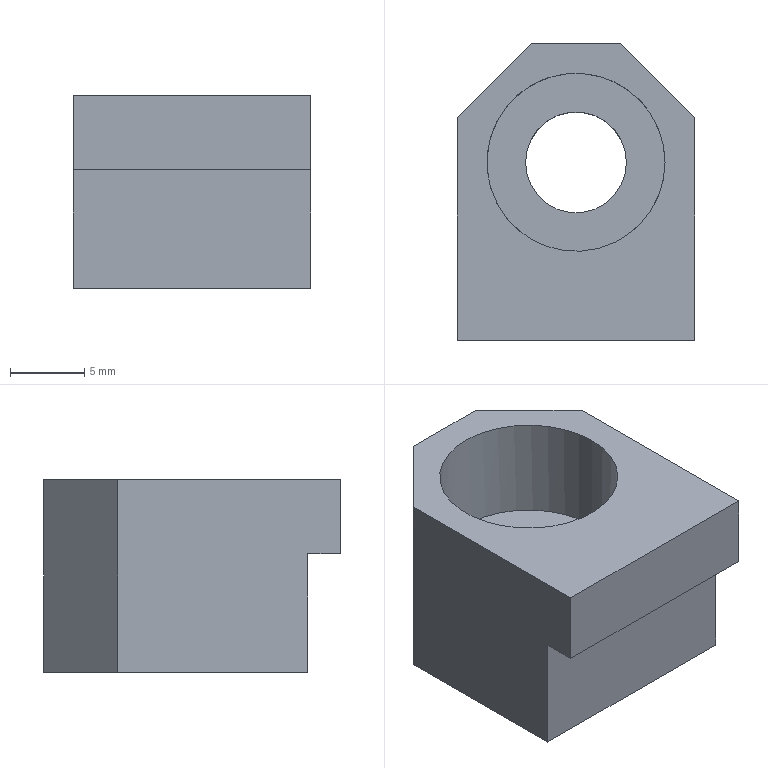Part | NX | features LIN_SOLID_COLOR 2 | 1 solid | 13 faces | box 16 x 20 x 13 mm | volume 2544 mm3 | plane 11 | cylinder 2 | commonest cylinder face diameters 6.8 x1 12 x1
STEP:
#1=CARTESIAN_POINT('',(-66.,111.5,-14.5));
#2=VERTEX_POINT('',#1);
#3=CARTESIAN_POINT('',(-66.,98.7,-14.5));
#4=VERTEX_POINT('',#3);
#5=CARTESIAN_POINT('',(-66.,106.,-14.5));
#6=DIRECTION('',(0.,-1.,0.));
#7=VECTOR('',#6,1000.);
#8=LINE('',#5,#7);
#9=EDGE_CURVE('',#2,#4,#8,.T.);
#10=ORIENTED_EDGE('',*,*,#9,.T.);
#11=CARTESIAN_POINT('',(-82.,98.7,-14.5));
#12=VERTEX_POINT('',#11);
#13=CARTESIAN_POINT('',(-78.,98.7,-14.5));
#14=DIRECTION('',(-1.,0.,0.));
#15=VECTOR('',#14,1000.);
#16=LINE('',#13,#15);
#17=EDGE_CURVE('',#4,#12,#16,.T.);
#18=ORIENTED_EDGE('',*,*,#17,.T.);
#19=CARTESIAN_POINT('',(-82.,111.5,-14.5));
#20=VERTEX_POINT('',#19);
#21=CARTESIAN_POINT('',(-82.,106.,-14.5));
#22=DIRECTION('',(0.,1.,0.));
#23=VECTOR('',#22,1000.);
#24=LINE('',#21,#23);
#25=EDGE_CURVE('',#12,#20,#24,.T.);
#26=ORIENTED_EDGE('',*,*,#25,.T.);
#27=CARTESIAN_POINT('',(-77.,116.5,-14.5));
#28=VERTEX_POINT('',#27);
#29=CARTESIAN_POINT('',(-82.75,110.75,-14.5));
#30=DIRECTION('',(0.7071,0.7071,0.));
#31=VECTOR('',#30,1000.);
#32=LINE('',#29,#31);
#33=EDGE_CURVE('',#28,#20,#32,.F.);
#34=ORIENTED_EDGE('',*,*,#33,.F.);
#35=CARTESIAN_POINT('',(-71.,116.5,-14.5));
#36=VERTEX_POINT('',#35);
#37=CARTESIAN_POINT('',(-78.,116.5,-14.5));
#38=DIRECTION('',(1.,0.,0.));
#39=VECTOR('',#38,1000.);
#40=LINE('',#37,#39);
#41=EDGE_CURVE('',#28,#36,#40,.T.);
#42=ORIENTED_EDGE('',*,*,#41,.T.);
#43=CARTESIAN_POINT('',(-69.25,114.75,-14.5));
#44=DIRECTION('',(0.7071,-0.7071,0.));
#45=VECTOR('',#44,1000.);
#46=LINE('',#43,#45);
#47=EDGE_CURVE('',#2,#36,#46,.F.);
#48=ORIENTED_EDGE('',*,*,#47,.F.);
#49=EDGE_LOOP('',(#10,#18,#26,#34,#42,#48));
#50=FACE_BOUND('',#49,.T.);
#51=CARTESIAN_POINT('',(-77.4,108.5,-14.5));
#52=VERTEX_POINT('',#51);
#53=CARTESIAN_POINT('',(-74.,108.5,-14.5));
#54=DIRECTION('',(0.,0.,-1.));
#55=DIRECTION('',(-1.,0.,0.));
#56=AXIS2_PLACEMENT_3D('',#53,#54,#55);
#57=CIRCLE('',#56,3.4);
#58=EDGE_CURVE('',#52,#52,#57,.F.);
#59=ORIENTED_EDGE('',*,*,#58,.T.);
#60=EDGE_LOOP('',(#59));
#61=FACE_BOUND('',#60,.T.);
#62=CARTESIAN_POINT('',(-78.,106.,-14.5));
#63=DIRECTION('',(0.,0.,-1.));
#64=DIRECTION('',(-1.,0.,0.));
#65=AXIS2_PLACEMENT_3D('',#62,#63,#64);
#66=PLANE('',#65);
#67=ADVANCED_FACE('',(#50,#61),#66,.T.);
#68=CARTESIAN_POINT('',(-82.,98.7,-6.5));
#69=VERTEX_POINT('',#68);
#70=CARTESIAN_POINT('',(-82.,98.7,-16.5));
#71=DIRECTION('',(0.,0.,1.));
#72=VECTOR('',#71,1000.);
#73=LINE('',#70,#72);
#74=EDGE_CURVE('',#12,#69,#73,.T.);
#75=ORIENTED_EDGE('',*,*,#74,.F.);
#76=ORIENTED_EDGE('',*,*,#17,.F.);
#77=CARTESIAN_POINT('',(-66.,98.7,-6.5));
#78=VERTEX_POINT('',#77);
#79=CARTESIAN_POINT('',(-66.,98.7,-16.5));
#80=DIRECTION('',(0.,0.,1.));
#81=VECTOR('',#80,1000.);
#82=LINE('',#79,#81);
#83=EDGE_CURVE('',#4,#78,#82,.T.);
#84=ORIENTED_EDGE('',*,*,#83,.T.);
#85=CARTESIAN_POINT('',(-82.,98.7,-6.5));
#86=DIRECTION('',(1.,0.,0.));
#87=VECTOR('',#86,1000.);
#88=LINE('',#85,#87);
#89=EDGE_CURVE('',#69,#78,#88,.T.);
#90=ORIENTED_EDGE('',*,*,#89,.F.);
#91=EDGE_LOOP('',(#75,#76,#84,#90));
#92=FACE_BOUND('',#91,.T.);
#93=CARTESIAN_POINT('',(-78.,98.7,-16.5));
#94=DIRECTION('',(0.,-1.,0.));
#95=DIRECTION('',(0.,0.,1.));
#96=AXIS2_PLACEMENT_3D('',#93,#94,#95);
#97=PLANE('',#96);
#98=ADVANCED_FACE('',(#92),#97,.T.);
#99=CARTESIAN_POINT('',(-66.,96.5,-1.5));
#100=VERTEX_POINT('',#99);
#101=CARTESIAN_POINT('',(-66.,111.5,-1.5));
#102=VERTEX_POINT('',#101);
#103=CARTESIAN_POINT('',(-66.,106.,-1.5));
#104=DIRECTION('',(0.,1.,0.));
#105=VECTOR('',#104,1000.);
#106=LINE('',#103,#105);
#107=EDGE_CURVE('',#100,#102,#106,.T.);
#108=ORIENTED_EDGE('',*,*,#107,.F.);
#109=CARTESIAN_POINT('',(-66.,96.5,-6.5));
#110=VERTEX_POINT('',#109);
#111=CARTESIAN_POINT('',(-66.,96.5,-16.5));
#112=DIRECTION('',(0.,0.,1.));
#113=VECTOR('',#112,1000.);
#114=LINE('',#111,#113);
#115=EDGE_CURVE('',#110,#100,#114,.T.);
#116=ORIENTED_EDGE('',*,*,#115,.F.);
#117=CARTESIAN_POINT('',(-66.,106.,-6.5));
#118=DIRECTION('',(0.,1.,0.));
#119=VECTOR('',#118,1000.);
#120=LINE('',#117,#119);
#121=EDGE_CURVE('',#110,#78,#120,.T.);
#122=ORIENTED_EDGE('',*,*,#121,.T.);
#123=ORIENTED_EDGE('',*,*,#83,.F.);
#124=ORIENTED_EDGE('',*,*,#9,.F.);
#125=CARTESIAN_POINT('',(-66.,111.5,-16.5));
#126=DIRECTION('',(0.,0.,-1.));
#127=VECTOR('',#126,1000.);
#128=LINE('',#125,#127);
#129=EDGE_CURVE('',#102,#2,#128,.T.);
#130=ORIENTED_EDGE('',*,*,#129,.F.);
#131=EDGE_LOOP('',(#108,#116,#122,#123,#124,#130));
#132=FACE_BOUND('',#131,.T.);
#133=CARTESIAN_POINT('',(-66.,106.,-16.5));
#134=DIRECTION('',(1.,0.,0.));
#135=DIRECTION('',(0.,0.,-1.));
#136=AXIS2_PLACEMENT_3D('',#133,#134,#135);
#137=PLANE('',#136);
#138=ADVANCED_FACE('',(#132),#137,.T.);
#139=ORIENTED_EDGE('',*,*,#41,.F.);
#140=CARTESIAN_POINT('',(-77.,116.5,-1.5));
#141=VERTEX_POINT('',#140);
#142=CARTESIAN_POINT('',(-77.,116.5,-16.5));
#143=DIRECTION('',(0.,0.,-1.));
#144=VECTOR('',#143,1000.);
#145=LINE('',#142,#144);
#146=EDGE_CURVE('',#141,#28,#145,.T.);
#147=ORIENTED_EDGE('',*,*,#146,.F.);
#148=CARTESIAN_POINT('',(-71.,116.5,-1.5));
#149=VERTEX_POINT('',#148);
#150=CARTESIAN_POINT('',(-78.,116.5,-1.5));
#151=DIRECTION('',(-1.,0.,0.));
#152=VECTOR('',#151,1000.);
#153=LINE('',#150,#152);
#154=EDGE_CURVE('',#149,#141,#153,.T.);
#155=ORIENTED_EDGE('',*,*,#154,.F.);
#156=CARTESIAN_POINT('',(-71.,116.5,-16.5));
#157=DIRECTION('',(0.,0.,1.));
#158=VECTOR('',#157,1000.);
#159=LINE('',#156,#158);
#160=EDGE_CURVE('',#36,#149,#159,.T.);
#161=ORIENTED_EDGE('',*,*,#160,.F.);
#162=EDGE_LOOP('',(#139,#147,#155,#161));
#163=FACE_BOUND('',#162,.T.);
#164=CARTESIAN_POINT('',(-78.,116.5,-16.5));
#165=DIRECTION('',(0.,1.,0.));
#166=DIRECTION('',(0.,0.,-1.));
#167=AXIS2_PLACEMENT_3D('',#164,#165,#166);
#168=PLANE('',#167);
#169=ADVANCED_FACE('',(#163),#168,.T.);
#170=ORIENTED_EDGE('',*,*,#25,.F.);
#171=ORIENTED_EDGE('',*,*,#74,.T.);
#172=CARTESIAN_POINT('',(-82.,96.5,-6.5));
#173=VERTEX_POINT('',#172);
#174=CARTESIAN_POINT('',(-82.,106.,-6.5));
#175=DIRECTION('',(0.,-1.,0.));
#176=VECTOR('',#175,1000.);
#177=LINE('',#174,#176);
#178=EDGE_CURVE('',#69,#173,#177,.T.);
#179=ORIENTED_EDGE('',*,*,#178,.T.);
#180=CARTESIAN_POINT('',(-82.,96.5,-1.5));
#181=VERTEX_POINT('',#180);
#182=CARTESIAN_POINT('',(-82.,96.5,-16.5));
#183=DIRECTION('',(0.,0.,1.));
#184=VECTOR('',#183,1000.);
#185=LINE('',#182,#184);
#186=EDGE_CURVE('',#173,#181,#185,.T.);
#187=ORIENTED_EDGE('',*,*,#186,.T.);
#188=CARTESIAN_POINT('',(-82.,111.5,-1.5));
#189=VERTEX_POINT('',#188);
#190=CARTESIAN_POINT('',(-82.,106.,-1.5));
#191=DIRECTION('',(0.,-1.,0.));
#192=VECTOR('',#191,1000.);
#193=LINE('',#190,#192);
#194=EDGE_CURVE('',#189,#181,#193,.T.);
#195=ORIENTED_EDGE('',*,*,#194,.F.);
#196=CARTESIAN_POINT('',(-82.,111.5,-16.5));
#197=DIRECTION('',(0.,0.,1.));
#198=VECTOR('',#197,1000.);
#199=LINE('',#196,#198);
#200=EDGE_CURVE('',#20,#189,#199,.T.);
#201=ORIENTED_EDGE('',*,*,#200,.F.);
#202=EDGE_LOOP('',(#170,#171,#179,#187,#195,#201));
#203=FACE_BOUND('',#202,.T.);
#204=CARTESIAN_POINT('',(-82.,106.,-16.5));
#205=DIRECTION('',(-1.,0.,0.));
#206=DIRECTION('',(0.,0.,1.));
#207=AXIS2_PLACEMENT_3D('',#204,#205,#206);
#208=PLANE('',#207);
#209=ADVANCED_FACE('',(#203),#208,.T.);
#210=CARTESIAN_POINT('',(-78.,96.5,-6.5));
#211=DIRECTION('',(1.,0.,0.));
#212=VECTOR('',#211,1000.);
#213=LINE('',#210,#212);
#214=EDGE_CURVE('',#173,#110,#213,.T.);
#215=ORIENTED_EDGE('',*,*,#214,.T.);
#216=ORIENTED_EDGE('',*,*,#115,.T.);
#217=CARTESIAN_POINT('',(-78.,96.5,-1.5));
#218=DIRECTION('',(1.,0.,0.));
#219=VECTOR('',#218,1000.);
#220=LINE('',#217,#219);
#221=EDGE_CURVE('',#181,#100,#220,.T.);
#222=ORIENTED_EDGE('',*,*,#221,.F.);
#223=ORIENTED_EDGE('',*,*,#186,.F.);
#224=EDGE_LOOP('',(#215,#216,#222,#223));
#225=FACE_BOUND('',#224,.T.);
#226=CARTESIAN_POINT('',(-78.,96.5,-16.5));
#227=DIRECTION('',(0.,-1.,0.));
#228=DIRECTION('',(0.,0.,1.));
#229=AXIS2_PLACEMENT_3D('',#226,#227,#228);
#230=PLANE('',#229);
#231=ADVANCED_FACE('',(#225),#230,.T.);
#232=CARTESIAN_POINT('',(-68.,108.5,-1.5));
#233=VERTEX_POINT('',#232);
#234=CARTESIAN_POINT('',(-74.,108.5,-1.5));
#235=DIRECTION('',(0.,0.,1.));
#236=DIRECTION('',(1.,0.,0.));
#237=AXIS2_PLACEMENT_3D('',#234,#235,#236);
#238=CIRCLE('',#237,6.);
#239=EDGE_CURVE('',#233,#233,#238,.T.);
#240=ORIENTED_EDGE('',*,*,#239,.F.);
#241=EDGE_LOOP('',(#240));
#242=FACE_BOUND('',#241,.T.);
#243=ORIENTED_EDGE('',*,*,#154,.T.);
#244=CARTESIAN_POINT('',(-82.75,110.75,-1.5));
#245=DIRECTION('',(-0.7071,-0.7071,0.));
#246=VECTOR('',#245,1000.);
#247=LINE('',#244,#246);
#248=EDGE_CURVE('',#189,#141,#247,.F.);
#249=ORIENTED_EDGE('',*,*,#248,.F.);
#250=ORIENTED_EDGE('',*,*,#194,.T.);
#251=ORIENTED_EDGE('',*,*,#221,.T.);
#252=ORIENTED_EDGE('',*,*,#107,.T.);
#253=CARTESIAN_POINT('',(-69.25,114.75,-1.5));
#254=DIRECTION('',(-0.7071,0.7071,0.));
#255=VECTOR('',#254,1000.);
#256=LINE('',#253,#255);
#257=EDGE_CURVE('',#149,#102,#256,.F.);
#258=ORIENTED_EDGE('',*,*,#257,.F.);
#259=EDGE_LOOP('',(#243,#249,#250,#251,#252,#258));
#260=FACE_BOUND('',#259,.T.);
#261=CARTESIAN_POINT('',(-78.,106.,-1.5));
#262=DIRECTION('',(0.,0.,1.));
#263=DIRECTION('',(1.,0.,0.));
#264=AXIS2_PLACEMENT_3D('',#261,#262,#263);
#265=PLANE('',#264);
#266=ADVANCED_FACE('',(#242,#260),#265,.T.);
#267=ORIENTED_EDGE('',*,*,#89,.T.);
#268=ORIENTED_EDGE('',*,*,#121,.F.);
#269=ORIENTED_EDGE('',*,*,#214,.F.);
#270=ORIENTED_EDGE('',*,*,#178,.F.);
#271=EDGE_LOOP('',(#267,#268,#269,#270));
#272=FACE_BOUND('',#271,.T.);
#273=CARTESIAN_POINT('',(-82.,98.5,-6.5));
#274=DIRECTION('',(0.,0.,1.));
#275=DIRECTION('',(1.,0.,0.));
#276=AXIS2_PLACEMENT_3D('',#273,#274,#275);
#277=PLANE('',#276);
#278=ADVANCED_FACE('',(#272),#277,.F.);
#279=ORIENTED_EDGE('',*,*,#33,.T.);
#280=ORIENTED_EDGE('',*,*,#200,.T.);
#281=ORIENTED_EDGE('',*,*,#248,.T.);
#282=ORIENTED_EDGE('',*,*,#146,.T.);
#283=EDGE_LOOP('',(#279,#280,#281,#282));
#284=FACE_BOUND('',#283,.T.);
#285=CARTESIAN_POINT('',(-82.,111.5,-16.5));
#286=DIRECTION('',(0.7071,-0.7071,0.));
#287=DIRECTION('',(-0.7071,-0.7071,0.));
#288=AXIS2_PLACEMENT_3D('',#285,#286,#287);
#289=PLANE('',#288);
#290=ADVANCED_FACE('',(#284),#289,.F.);
#291=ORIENTED_EDGE('',*,*,#47,.T.);
#292=ORIENTED_EDGE('',*,*,#160,.T.);
#293=ORIENTED_EDGE('',*,*,#257,.T.);
#294=ORIENTED_EDGE('',*,*,#129,.T.);
#295=EDGE_LOOP('',(#291,#292,#293,#294));
#296=FACE_BOUND('',#295,.T.);
#297=CARTESIAN_POINT('',(-71.,116.5,-16.5));
#298=DIRECTION('',(-0.7071,-0.7071,0.));
#299=DIRECTION('',(-0.7071,0.7071,0.));
#300=AXIS2_PLACEMENT_3D('',#297,#298,#299);
#301=PLANE('',#300);
#302=ADVANCED_FACE('',(#296),#301,.F.);
#303=CARTESIAN_POINT('',(-77.4,108.5,-8.5));
#304=VERTEX_POINT('',#303);
#305=CARTESIAN_POINT('',(-74.,108.5,-8.5));
#306=DIRECTION('',(0.,0.,-1.));
#307=DIRECTION('',(-1.,0.,0.));
#308=AXIS2_PLACEMENT_3D('',#305,#306,#307);
#309=CIRCLE('',#308,3.4);
#310=EDGE_CURVE('',#304,#304,#309,.F.);
#311=ORIENTED_EDGE('',*,*,#310,.T.);
#312=EDGE_LOOP('',(#311));
#313=FACE_BOUND('',#312,.T.);
#314=ORIENTED_EDGE('',*,*,#58,.F.);
#315=EDGE_LOOP('',(#314));
#316=FACE_BOUND('',#315,.T.);
#317=CARTESIAN_POINT('',(-74.,108.5,-14.5));
#318=DIRECTION('',(0.,0.,1.));
#319=DIRECTION('',(1.,0.,0.));
#320=AXIS2_PLACEMENT_3D('',#317,#318,#319);
#321=CYLINDRICAL_SURFACE('',#320,3.4);
#322=ADVANCED_FACE('',(#313,#316),#321,.F.);
#323=CARTESIAN_POINT('',(-80.,108.5,-8.5));
#324=VERTEX_POINT('',#323);
#325=CARTESIAN_POINT('',(-74.,108.5,-8.5));
#326=DIRECTION('',(0.,0.,-1.));
#327=DIRECTION('',(-1.,0.,0.));
#328=AXIS2_PLACEMENT_3D('',#325,#326,#327);
#329=CIRCLE('',#328,6.);
#330=EDGE_CURVE('',#324,#324,#329,.T.);
#331=ORIENTED_EDGE('',*,*,#330,.F.);
#332=EDGE_LOOP('',(#331));
#333=FACE_BOUND('',#332,.T.);
#334=ORIENTED_EDGE('',*,*,#310,.F.);
#335=EDGE_LOOP('',(#334));
#336=FACE_BOUND('',#335,.T.);
#337=CARTESIAN_POINT('',(-74.,108.5,-8.5));
#338=DIRECTION('',(0.,0.,-1.));
#339=DIRECTION('',(-1.,0.,0.));
#340=AXIS2_PLACEMENT_3D('',#337,#338,#339);
#341=PLANE('',#340);
#342=ADVANCED_FACE('',(#333,#336),#341,.F.);
#343=ORIENTED_EDGE('',*,*,#239,.T.);
#344=EDGE_LOOP('',(#343));
#345=FACE_BOUND('',#344,.T.);
#346=ORIENTED_EDGE('',*,*,#330,.T.);
#347=EDGE_LOOP('',(#346));
#348=FACE_BOUND('',#347,.T.);
#349=CARTESIAN_POINT('',(-74.,108.5,5.5));
#350=DIRECTION('',(0.,0.,1.));
#351=DIRECTION('',(1.,0.,0.));
#352=AXIS2_PLACEMENT_3D('',#349,#350,#351);
#353=CYLINDRICAL_SURFACE('',#352,6.);
#354=ADVANCED_FACE('',(#345,#348),#353,.F.);
#355=CLOSED_SHELL('',(#67,#98,#138,#169,#209,#231,#266,#278,#290,#302,#322,#342,#354));
#356=MANIFOLD_SOLID_BREP('',#355);
#357=(LENGTH_UNIT()NAMED_UNIT(*)SI_UNIT(.MILLI.,.METRE.));
#358=UNCERTAINTY_MEASURE_WITH_UNIT(LENGTH_MEASURE(0.00001),#357,'','');
#359=(NAMED_UNIT(*)PLANE_ANGLE_UNIT()SI_UNIT($,.RADIAN.));
#360=(NAMED_UNIT(*)SI_UNIT($,.STERADIAN.)SOLID_ANGLE_UNIT());
#361=(GEOMETRIC_REPRESENTATION_CONTEXT(3)GLOBAL_UNCERTAINTY_ASSIGNED_CONTEXT((#358))GLOBAL_UNIT_ASSIGNED_CONTEXT((#357,#359,#360))REPRESENTATION_CONTEXT('',''));
#362=ADVANCED_BREP_SHAPE_REPRESENTATION('',(#356),#361);